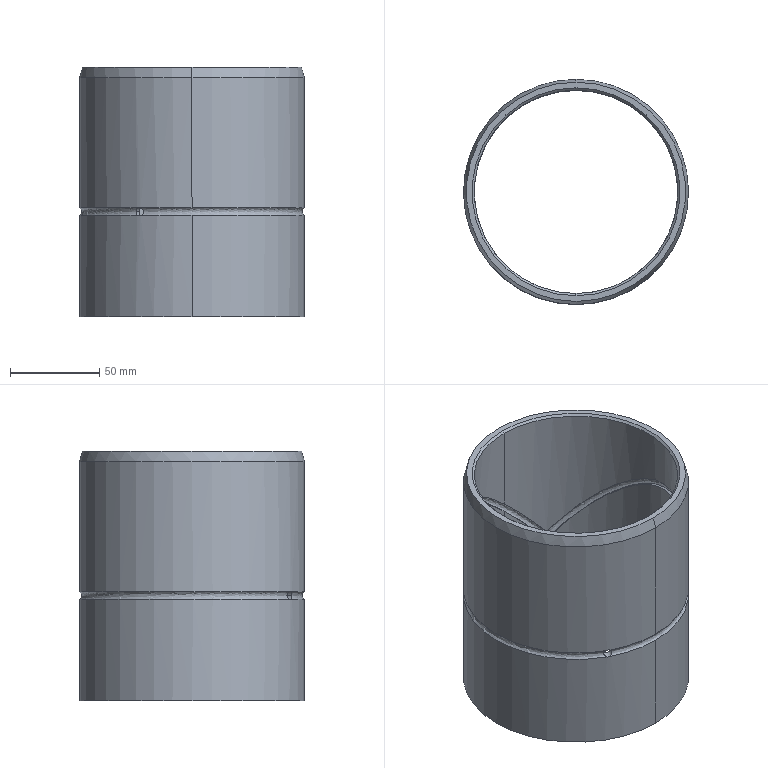Part | SolidWorks | features BaseBody 1, ICE 1, Scale 1 | 1 solid | 38 faces | box 126 x 126 x 140 mm | volume 308538 mm3 | spline 16 | cylinder 16 | cone 4 | plane 2 | commonest cylinder face diameters 114 x8 4.8 x4 126 x4